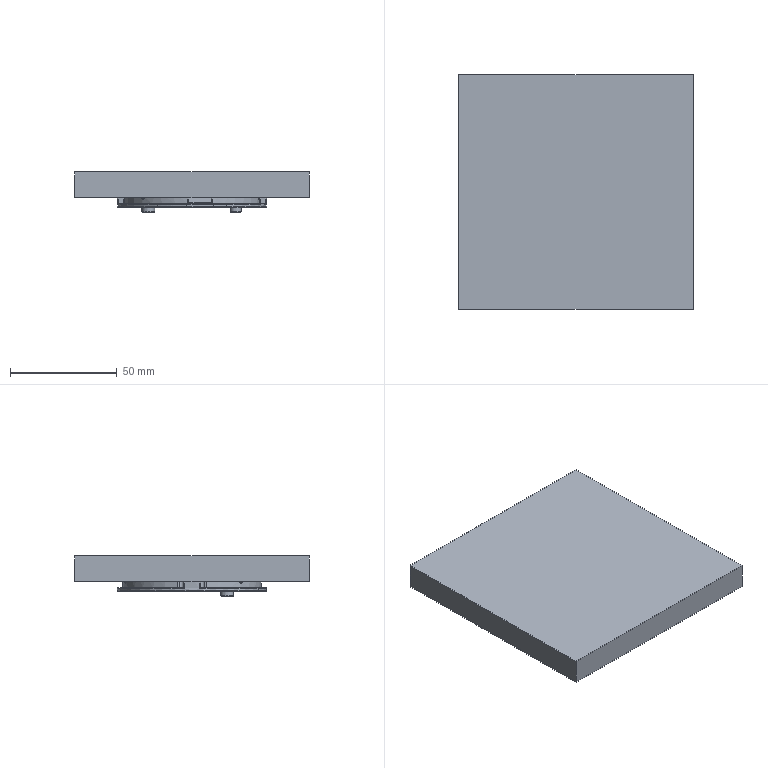NC program | NX | posted with a generic post | part box 110 x 110 x 18.8 mm
Lines 3402 to 4286 of 9447:
(CAVITY_MILL_COPY_1_COPY , TOOL : D3)
N6784 T17 M6
N6786 G54
N6788 G17 G0 G90 X-34.29 Y3.742 S9500 M3
N6790 G43 Z30. H17
N6792 Z-4.25
N6794 G94 G1 Z-5.25 F1000.
N6796 G3 X-33.488 Y4.304 R1.
N6798 G2 X-32.872 Y5.112 R2.5 F1100.
N6800 X-33.214 Y6.069 R2.5
N6802 G3 X-33.807 Y6.848 R1.
N6804 G1 Z-4.25
N6806 G0 X-34.29 Y3.742 Z-4.5
N6808 G1 Z-5.5 F1000.
N6810 G3 X-33.488 Y4.304 R1.
N6812 G2 X-32.872 Y5.112 R2.5 F1100.
N6814 X-33.214 Y6.069 R2.5
N6816 G3 X-33.807 Y6.848 R1.
N6818 G1 Z-4.5
N6820 G0 X-34.29 Y3.742 Z-4.75
N6822 G1 Z-5.75 F1000.
N6824 G3 X-33.488 Y4.304 R1.
N6826 G2 X-32.872 Y5.112 R2.5 F1100.
N6828 X-33.214 Y6.069 R2.5
N6830 G3 X-33.807 Y6.848 R1.
N6832 G1 Z-4.75
N6834 G0 X-34.29 Y3.742 Z-5.
N6836 G1 Z-6. F1000.
N6838 G3 X-33.488 Y4.304 R1.
N6840 G2 X-32.872 Y5.112 R2.5 F1100.
N6842 X-33.214 Y6.069 R2.5
N6844 G3 X-33.807 Y6.848 R1.
N6846 G1 Z-5.
N6848 G0 X-34.29 Y3.742 Z-5.25
N6850 G1 Z-6.25 F1000.
N6852 G3 X-33.488 Y4.304 R1.
N6854 G2 X-32.872 Y5.112 R2.5 F1100.
N6856 X-33.214 Y6.069 R2.5
N6858 G3 X-33.807 Y6.848 R1.
N6860 G1 Z-5.25
N6862 G0 X-34.29 Y3.742 Z-5.5
N6864 G1 Z-6.5 F1000.
N6866 G3 X-33.488 Y4.304 R1.
N6868 G2 X-32.872 Y5.112 R2.5 F1100.
N6870 X-33.214 Y6.069 R2.5
N6872 G3 X-33.807 Y6.848 R1.
N6874 G1 Z-5.5
N6876 G0 X-34.29 Y3.742 Z-5.75
N6878 G1 Z-6.75 F1000.
N6880 G3 X-33.488 Y4.304 R1.
N6882 G2 X-32.872 Y5.112 R2.5 F1100.
N6884 X-33.214 Y6.069 R2.5
N6886 G3 X-33.807 Y6.848 R1.
N6888 G1 Z-5.75
N6890 G0 X-34.29 Y3.742 Z-6.
N6892 G1 Z-7. F1000.
N6894 G3 X-33.488 Y4.304 R1.
N6896 G2 X-32.872 Y5.112 R2.5 F1100.
N6898 X-33.214 Y6.069 R2.5
N6900 G3 X-33.807 Y6.848 R1.
N6902 G1 Z-6.
N6904 G0 X-34.29 Y3.742 Z-6.25
N6906 G1 Z-7.25 F1000.
N6908 G3 X-33.488 Y4.304 R1.
N6910 G2 X-32.872 Y5.112 R2.5 F1100.
N6912 X-33.214 Y6.069 R2.5
N6914 G3 X-33.807 Y6.848 R1.
N6916 G1 Z-6.25
N6918 G0 X-34.29 Y3.742 Z-6.5
N6920 G1 Z-7.5 F1000.
N6922 G3 X-33.488 Y4.304 R1.
N6924 G2 X-32.872 Y5.112 R2.5 F1100.
N6926 X-33.214 Y6.069 R2.5
N6928 G3 X-33.807 Y6.848 R1.
N6930 G1 Z-6.5
N6932 G0 X-34.29 Y3.742 Z-6.75
N6934 G1 Z-7.75 F1000.
N6936 G3 X-33.488 Y4.304 R1.
N6938 G2 X-32.872 Y5.112 R2.5 F1100.
N6940 X-33.214 Y6.069 R2.5
N6942 G3 X-33.807 Y6.848 R1.
N6944 G1 Z-6.75
N6946 G0 X-34.29 Y3.742 Z-7.
N6948 G1 Z-8. F1000.
N6950 G3 X-33.488 Y4.304 R1.
N6952 G2 X-32.872 Y5.112 R2.5 F1100.
N6954 X-33.214 Y6.069 R2.5
N6956 G3 X-33.807 Y6.848 R1.
N6958 G1 Z-7.
N6960 G0 X-34.29 Y3.742 Z-7.25
N6962 G1 Z-8.25 F1000.
N6964 G3 X-33.488 Y4.304 R1.
N6966 G2 X-32.872 Y5.112 R2.5 F1100.
N6968 X-33.214 Y6.069 R2.5
N6970 G3 X-33.807 Y6.848 R1.
N6972 G1 Z-7.25
N6974 G0 X-34.29 Y3.742 Z-7.5
N6976 G1 Z-8.5 F1000.
N6978 G3 X-33.488 Y4.304 R1.
N6980 G2 X-32.872 Y5.112 R2.5 F1100.
N6982 X-33.214 Y6.069 R2.5
N6984 G3 X-33.807 Y6.848 R1.
N6986 G1 Z-7.5
N6988 G0 X-34.29 Y3.742 Z-7.75
N6990 G1 Z-8.75 F1000.
N6992 G3 X-33.488 Y4.304 R1.
N6994 G2 X-32.872 Y5.112 R2.5 F1100.
N6996 X-33.214 Y6.069 R2.5
N6998 G3 X-33.807 Y6.848 R1.
N7000 G1 Z-7.75
N7002 G0 X-34.29 Y3.742 Z-8.
N7004 G1 Z-9. F1000.
N7006 G3 X-33.488 Y4.304 R1.
N7008 G2 X-32.872 Y5.112 R2.5 F1100.
N7010 X-33.214 Y6.069 R2.5
N7012 G3 X-33.807 Y6.848 R1.
N7014 G1 Z-8.
N7016 G0 X-35.784 Y5.65 Z-8.25
N7018 G1 Z-9.25 F1000.
N7020 G3 X-34.851 Y5.429 R1.
N7022 G2 X-34.322 Y5.5 R2. F1100.
N7024 G1 X-33.065
N7026 G2 X-33.185 Y6.925 R2.5
N7028 G1 X-33.147 Y7.106
N7030 G3 X-33.454 Y8.058 R1.
N7032 G1 X-33.529 Y8.126
N7034 Z-8.25
N7036 G0 X-35.784 Y5.65 Z-8.5
N7038 G1 Z-9.5 F1000.
N7040 G3 X-34.851 Y5.429 R1.
N7042 G2 X-34.322 Y5.5 R2. F1100.
N7044 G1 X-33.065
N7046 G2 X-33.185 Y6.925 R2.5
N7048 G1 X-33.147 Y7.106
N7050 G3 X-33.454 Y8.058 R1.
N7052 G1 X-33.529 Y8.126
N7054 Z-8.5
N7056 G0 X-35.784 Y5.65 Z-8.75
N7058 G1 Z-9.75 F1000.
N7060 G3 X-34.851 Y5.429 R1.
N7062 G2 X-34.322 Y5.5 R2. F1100.
N7064 G1 X-33.065
N7066 G2 X-33.185 Y6.925 R2.5
N7068 G1 X-33.147 Y7.106
N7070 G3 X-33.454 Y8.058 R1.
N7072 G1 X-33.529 Y8.126
N7074 Z-8.75
N7076 G0 X-35.784 Y5.65 Z-9.
N7078 G1 Z-10. F1000.
N7080 G3 X-34.851 Y5.429 R1.
N7082 G2 X-34.322 Y5.5 R2. F1100.
N7084 G1 X-33.065
N7086 G2 X-33.185 Y6.925 R2.5
N7088 G1 X-33.147 Y7.106
N7090 G3 X-33.454 Y8.058 R1.
N7092 G1 X-33.529 Y8.126
N7094 Z-9.
N7096 G0 X-35.784 Y5.65 Z-9.25
N7098 G1 Z-10.25 F1000.
N7100 G3 X-34.851 Y5.429 R1.
N7102 G2 X-34.322 Y5.5 R2. F1100.
N7104 G1 X-33.065
N7106 G2 X-33.185 Y6.925 R2.5
N7108 G1 X-33.147 Y7.106
N7110 G3 X-33.454 Y8.058 R1.
N7112 G1 X-33.529 Y8.126
N7114 Z-9.25
N7116 G0 X-35.784 Y5.65 Z-9.5
N7118 G1 Z-10.5 F1000.
N7120 G3 X-34.851 Y5.429 R1.
N7122 G2 X-34.322 Y5.5 R2. F1100.
N7124 G1 X-33.065
N7126 G2 X-33.185 Y6.925 R2.5
N7128 G1 X-33.147 Y7.106
N7130 G3 X-33.454 Y8.058 R1.
N7132 G1 X-33.529 Y8.126
N7134 Z-9.5
N7136 G0 X-35.784 Y5.65 Z-9.75
N7138 G1 Z-10.75 F1000.
N7140 G3 X-34.851 Y5.429 R1.
N7142 G2 X-34.322 Y5.5 R2. F1100.
N7144 G1 X-33.065
N7146 G2 X-33.185 Y6.925 R2.5
N7148 G1 X-33.147 Y7.106
N7150 G3 X-33.454 Y8.058 R1.
N7152 G1 X-33.529 Y8.126
N7154 Z-9.75
N7156 G0 X-35.784 Y5.65 Z-10.
N7158 G1 Z-11. F1000.
N7160 G3 X-34.851 Y5.429 R1.
N7162 G2 X-34.322 Y5.5 R2. F1100.
N7164 G1 X-33.065
N7166 G2 X-33.185 Y6.925 R2.5
N7168 G1 X-33.147 Y7.106
N7170 G3 X-33.454 Y8.058 R1.
N7172 G1 X-33.529 Y8.126
N7174 Z-10.
N7176 G0 X-35.784 Y5.65 Z-10.25
N7178 G1 Z-11.25 F1000.
N7180 G3 X-34.851 Y5.429 R1.
N7182 G2 X-34.322 Y5.5 R2. F1100.
N7184 G1 X-33.065
N7186 G2 X-33.185 Y6.925 R2.5
N7188 G1 X-33.147 Y7.106
N7190 G3 X-33.454 Y8.058 R1.
N7192 G1 X-33.529 Y8.126
N7194 Z-10.25
N7196 G0 X-35.784 Y5.65 Z-10.5
N7198 G1 Z-11.5 F1000.
N7200 G3 X-34.851 Y5.429 R1.
N7202 G2 X-34.322 Y5.5 R2. F1100.
N7204 G1 X-33.065
N7206 G2 X-33.185 Y6.925 R2.5
N7208 G1 X-33.147 Y7.106
N7210 G3 X-33.454 Y8.058 R1.
N7212 G1 X-33.529 Y8.126
N7214 Z-10.5
N7216 G0 X-35.784 Y5.65 Z-10.75
N7218 G1 Z-11.75 F1000.
N7220 G3 X-34.851 Y5.429 R1.
N7222 G2 X-34.322 Y5.5 R2. F1100.
N7224 G1 X-33.065
N7226 G2 X-33.185 Y6.925 R2.5
N7228 G1 X-33.147 Y7.106
N7230 G3 X-33.454 Y8.058 R1.
N7232 G1 X-33.529 Y8.126
N7234 Z-10.75
N7236 G0 X-35.784 Y5.65 Z-11.
N7238 G1 Z-12. F1000.
N7240 G3 X-34.851 Y5.429 R1.
N7242 G2 X-34.322 Y5.5 R2. F1100.
N7244 G1 X-33.065
N7246 G2 X-33.185 Y6.925 R2.5
N7248 G1 X-33.147 Y7.106
N7250 G3 X-33.454 Y8.058 R1.
N7252 G1 X-33.529 Y8.126
N7254 Z-11.
N7256 G0 Z30.
N7258 X-33.807 Y-6.848
N7260 Z-4.25
N7262 G1 Z-5.25 F1000.
N7264 G3 X-33.214 Y-6.069 R1.
N7266 G2 X-32.872 Y-5.112 R2.5 F1100.
N7268 X-33.488 Y-4.304 R2.5
N7270 G3 X-34.29 Y-3.742 R1.
N7272 G1 Z-4.25
N7274 G0 X-33.807 Y-6.848 Z-4.5
N7276 G1 Z-5.5 F1000.
N7278 G3 X-33.214 Y-6.069 R1.
N7280 G2 X-32.872 Y-5.112 R2.5 F1100.
N7282 X-33.488 Y-4.304 R2.5
N7284 G3 X-34.29 Y-3.742 R1.
N7286 G1 Z-4.5
N7288 G0 X-33.807 Y-6.848 Z-4.75
N7290 G1 Z-5.75 F1000.
N7292 G3 X-33.214 Y-6.069 R1.
N7294 G2 X-32.872 Y-5.112 R2.5 F1100.
N7296 X-33.488 Y-4.304 R2.5
N7298 G3 X-34.29 Y-3.742 R1.
N7300 G1 Z-4.75
N7302 G0 X-33.807 Y-6.848 Z-5.
N7304 G1 Z-6. F1000.
N7306 G3 X-33.214 Y-6.069 R1.
N7308 G2 X-32.872 Y-5.112 R2.5 F1100.
N7310 X-33.488 Y-4.304 R2.5
N7312 G3 X-34.291 Y-3.741 R1.
N7314 G1 Z-5.
N7316 G0 X-33.807 Y-6.848 Z-5.25
N7318 G1 Z-6.25 F1000.
N7320 G3 X-33.214 Y-6.069 R1.
N7322 G2 X-32.872 Y-5.112 R2.5 F1100.
N7324 X-33.488 Y-4.304 R2.5
N7326 G3 X-34.29 Y-3.742 R1.
N7328 G1 Z-5.25
N7330 G0 X-33.807 Y-6.848 Z-5.5
N7332 G1 Z-6.5 F1000.
N7334 G3 X-33.214 Y-6.069 R1.
N7336 G2 X-32.872 Y-5.112 R2.5 F1100.
N7338 X-33.488 Y-4.304 R2.5
N7340 G3 X-34.29 Y-3.742 R1.
N7342 G1 Z-5.5
N7344 G0 X-33.807 Y-6.848 Z-5.75
N7346 G1 Z-6.75 F1000.
N7348 G3 X-33.214 Y-6.069 R1.
N7350 G2 X-32.872 Y-5.112 R2.5 F1100.
N7352 X-33.488 Y-4.304 R2.5
N7354 G3 X-34.29 Y-3.742 R1.
N7356 G1 Z-5.75
N7358 G0 X-33.807 Y-6.848 Z-6.
N7360 G1 Z-7. F1000.
N7362 G3 X-33.214 Y-6.069 R1.
N7364 G2 X-32.872 Y-5.112 R2.5 F1100.
N7366 X-33.488 Y-4.304 R2.5
N7368 G3 X-34.29 Y-3.742 R1.
N7370 G1 Z-6.
N7372 G0 X-33.807 Y-6.848 Z-6.25
N7374 G1 Z-7.25 F1000.
N7376 G3 X-33.214 Y-6.069 R1.
N7378 G2 X-32.872 Y-5.112 R2.5 F1100.
N7380 X-33.488 Y-4.304 R2.5
N7382 G3 X-34.29 Y-3.742 R1.
N7384 G1 Z-6.25
N7386 G0 X-33.807 Y-6.848 Z-6.5
N7388 G1 Z-7.5 F1000.
N7390 G3 X-33.214 Y-6.069 R1.
N7392 G2 X-32.872 Y-5.112 R2.5 F1100.
N7394 X-33.488 Y-4.304 R2.5
N7396 G3 X-34.29 Y-3.742 R1.
N7398 G1 Z-6.5
N7400 G0 X-33.807 Y-6.848 Z-6.75
N7402 G1 Z-7.75 F1000.
N7404 G3 X-33.214 Y-6.069 R1.
N7406 G2 X-32.872 Y-5.112 R2.5 F1100.
N7408 X-33.488 Y-4.304 R2.5
N7410 G3 X-34.29 Y-3.742 R1.
N7412 G1 Z-6.75
N7414 G0 X-33.807 Y-6.848 Z-7.
N7416 G1 Z-8. F1000.
N7418 G3 X-33.214 Y-6.069 R1.
N7420 G2 X-32.872 Y-5.112 R2.5 F1100.
N7422 X-33.488 Y-4.304 R2.5
N7424 G3 X-34.29 Y-3.742 R1.
N7426 G1 Z-7.
N7428 G0 X-33.807 Y-6.848 Z-7.25
N7430 G1 Z-8.25 F1000.
N7432 G3 X-33.214 Y-6.069 R1.
N7434 G2 X-32.872 Y-5.112 R2.5 F1100.
N7436 X-33.488 Y-4.304 R2.5
N7438 G3 X-34.29 Y-3.742 R1.
N7440 G1 Z-7.25
N7442 G0 X-33.807 Y-6.848 Z-7.5
N7444 G1 Z-8.5 F1000.
N7446 G3 X-33.214 Y-6.069 R1.
N7448 G2 X-32.872 Y-5.112 R2.5 F1100.
N7450 X-33.488 Y-4.304 R2.5
N7452 G3 X-34.29 Y-3.742 R1.
N7454 G1 Z-7.5
N7456 G0 X-33.807 Y-6.848 Z-7.75
N7458 G1 Z-8.75 F1000.
N7460 G3 X-33.214 Y-6.069 R1.
N7462 G2 X-32.872 Y-5.112 R2.5 F1100.
N7464 X-33.488 Y-4.304 R2.5
N7466 G3 X-34.29 Y-3.742 R1.
N7468 G1 Z-7.75
N7470 G0 X-33.807 Y-6.848 Z-8.
N7472 G1 Z-9. F1000.
N7474 G3 X-33.214 Y-6.069 R1.
N7476 G2 X-32.872 Y-5.112 R2.5 F1100.
N7478 X-33.488 Y-4.304 R2.5
N7480 G3 X-34.29 Y-3.741 R1.
N7482 G1 Z-8.
N7484 G0 X-33.529 Y-8.126 Z-8.25
N7486 G1 Z-9.25 F1000.
N7488 X-33.454 Y-8.058
N7490 G3 X-33.147 Y-7.106 R1.
N7492 G1 X-33.185 Y-6.925 F1100.
N7494 G2 X-33.065 Y-5.5 R2.5
N7496 G1 X-34.322
N7498 G2 X-34.851 Y-5.429 R2.
N7500 G3 X-35.784 Y-5.65 R1.
N7502 G1 Z-8.25
N7504 G0 X-33.529 Y-8.126 Z-8.5
N7506 G1 Z-9.5 F1000.
N7508 X-33.454 Y-8.058
N7510 G3 X-33.147 Y-7.106 R1.
N7512 G1 X-33.185 Y-6.925 F1100.
N7514 G2 X-33.065 Y-5.5 R2.5
N7516 G1 X-34.322
N7518 G2 X-34.851 Y-5.429 R2.
N7520 G3 X-35.784 Y-5.65 R1.
N7522 G1 Z-8.5
N7524 G0 X-33.529 Y-8.126 Z-8.75
N7526 G1 Z-9.75 F1000.
N7528 X-33.454 Y-8.058
N7530 G3 X-33.147 Y-7.106 R1.
N7532 G1 X-33.185 Y-6.925 F1100.
N7534 G2 X-33.065 Y-5.5 R2.5
N7536 G1 X-34.322
N7538 G2 X-34.851 Y-5.429 R2.
N7540 G3 X-35.784 Y-5.65 R1.
N7542 G1 Z-8.75
N7544 G0 X-33.529 Y-8.126 Z-9.
N7546 G1 Z-10. F1000.
N7548 X-33.454 Y-8.058
N7550 G3 X-33.147 Y-7.106 R1.
N7552 G1 X-33.185 Y-6.925 F1100.
N7554 G2 X-33.065 Y-5.5 R2.5
N7556 G1 X-34.322
N7558 G2 X-34.851 Y-5.429 R2.
N7560 G3 X-35.784 Y-5.65 R1.
N7562 G1 Z-9.
N7564 G0 X-33.529 Y-8.126 Z-9.25
N7566 G1 Z-10.25 F1000.
N7568 X-33.454 Y-8.058
N7570 G3 X-33.147 Y-7.106 R1.
N7572 G1 X-33.185 Y-6.925 F1100.
N7574 G2 X-33.065 Y-5.5 R2.5
N7576 G1 X-34.322
N7578 G2 X-34.851 Y-5.429 R2.
N7580 G3 X-35.784 Y-5.65 R1.
N7582 G1 Z-9.25
N7584 G0 X-33.529 Y-8.126 Z-9.5
N7586 G1 Z-10.5 F1000.
N7588 X-33.454 Y-8.058
N7590 G3 X-33.147 Y-7.106 R1.
N7592 G1 X-33.185 Y-6.925 F1100.
N7594 G2 X-33.065 Y-5.5 R2.5
N7596 G1 X-34.322
N7598 G2 X-34.851 Y-5.429 R2.
N7600 G3 X-35.784 Y-5.65 R1.
N7602 G1 Z-9.5
N7604 G0 X-33.529 Y-8.126 Z-9.75
N7606 G1 Z-10.75 F1000.
N7608 X-33.454 Y-8.058
N7610 G3 X-33.147 Y-7.106 R1.
N7612 G1 X-33.185 Y-6.925 F1100.
N7614 G2 X-33.065 Y-5.5 R2.5
N7616 G1 X-34.322
N7618 G2 X-34.851 Y-5.429 R2.
N7620 G3 X-35.784 Y-5.65 R1.
N7622 G1 Z-9.75
N7624 G0 X-33.529 Y-8.126 Z-10.
N7626 G1 Z-11. F1000.
N7628 X-33.454 Y-8.058
N7630 G3 X-33.147 Y-7.106 R1.
N7632 G1 X-33.185 Y-6.925 F1100.
N7634 G2 X-33.065 Y-5.5 R2.5
N7636 G1 X-34.322
N7638 G2 X-34.851 Y-5.429 R2.
N7640 G3 X-35.784 Y-5.65 R1.
N7642 G1 Z-10.
N7644 G0 X-33.529 Y-8.126 Z-10.25
N7646 G1 Z-11.25 F1000.
N7648 X-33.454 Y-8.058
N7650 G3 X-33.147 Y-7.106 R1.
N7652 G1 X-33.185 Y-6.925 F1100.
N7654 G2 X-33.065 Y-5.5 R2.5
N7656 G1 X-34.322
N7658 G2 X-34.851 Y-5.429 R2.
N7660 G3 X-35.784 Y-5.65 R1.
N7662 G1 Z-10.25
N7664 G0 X-33.529 Y-8.126 Z-10.5
N7666 G1 Z-11.5 F1000.
N7668 X-33.454 Y-8.058
N7670 G3 X-33.147 Y-7.106 R1.
N7672 G1 X-33.185 Y-6.925 F1100.
N7674 G2 X-33.065 Y-5.5 R2.5
N7676 G1 X-34.322
N7678 G2 X-34.851 Y-5.429 R2.
N7680 G3 X-35.784 Y-5.65 R1.
N7682 G1 Z-10.5
N7684 G0 X-33.529 Y-8.126 Z-10.75
N7686 G1 Z-11.75 F1000.
N7688 X-33.454 Y-8.058
N7690 G3 X-33.147 Y-7.106 R1.
N7692 G1 X-33.185 Y-6.925 F1100.
N7694 G2 X-33.065 Y-5.5 R2.5
N7696 G1 X-34.322
N7698 G2 X-34.851 Y-5.429 R2.
N7700 G3 X-35.784 Y-5.65 R1.
N7702 G1 Z-10.75
N7704 G0 X-33.529 Y-8.126 Z-11.
N7706 G1 Z-12. F1000.
N7708 X-33.454 Y-8.058
N7710 G3 X-33.147 Y-7.106 R1.
N7712 G1 X-33.185 Y-6.925 F1100.
N7714 G2 X-33.065 Y-5.5 R2.5
N7716 G1 X-34.322
N7718 G2 X-34.851 Y-5.429 R2.
N7720 G3 X-35.784 Y-5.65 R1.
N7722 G1 Z-11.
N7724 G0 Z30.
N7726 X-24.498 Y-14.169
N7728 Z-4.25
N7730 G1 Z-5.25 F1000.
N7732 X-24.56 Y-14.286
N7734 G3 X-24.527 Y-15.286 R1.
N7736 X-23.81 Y-16.379 R28.9 F1100.
N7738 G2 X-22.711 Y-16.183 R2.5
N7740 G3 X-21.835 Y-15.745 R1.
N7742 G1 Z-4.25
N7744 G0 X-24.498 Y-14.169 Z-4.5
N7746 G1 Z-5.5 F1000.
N7748 X-24.56 Y-14.286
N7750 G3 X-24.527 Y-15.286 R1.
N7752 X-23.81 Y-16.379 R28.9 F1100.
N7754 G2 X-22.711 Y-16.183 R2.5
N7756 G3 X-21.835 Y-15.745 R1.
N7758 G1 Z-4.5
N7760 G0 X-24.498 Y-14.169 Z-4.75
N7762 G1 Z-5.75 F1000.
N7764 X-24.56 Y-14.286
N7766 G3 X-24.527 Y-15.286 R1.
N7768 X-23.81 Y-16.379 R28.9 F1100.
N7770 G2 X-22.711 Y-16.183 R2.5
N7772 G3 X-21.835 Y-15.745 R1.
N7774 G1 Z-4.75
N7776 G0 X-24.498 Y-14.169 Z-5.
N7778 G1 Z-6. F1000.
N7780 X-24.56 Y-14.286
N7782 G3 X-24.527 Y-15.286 R1.
N7784 X-23.81 Y-16.379 R28.9 F1100.
N7786 G2 X-22.711 Y-16.183 R2.5
N7788 G3 X-21.835 Y-15.745 R1.
N7790 G1 Z-5.
N7792 G0 X-24.498 Y-14.169 Z-5.25
N7794 G1 Z-6.25 F1000.
N7796 X-24.56 Y-14.286
N7798 G3 X-24.527 Y-15.286 R1.
N7800 X-23.81 Y-16.379 R28.9 F1100.
N7802 G2 X-22.711 Y-16.183 R2.5
N7804 G3 X-21.835 Y-15.745 R1.
N7806 G1 Z-5.25
N7808 G0 X-24.498 Y-14.169 Z-5.5
N7810 G1 Z-6.5 F1000.
N7812 X-24.56 Y-14.286
N7814 G3 X-24.527 Y-15.286 R1.
N7816 X-23.81 Y-16.379 R28.9 F1100.
N7818 G2 X-22.711 Y-16.183 R2.5
N7820 G3 X-21.835 Y-15.745 R1.
N7822 G1 Z-5.5
N7824 G0 X-24.498 Y-14.169 Z-5.75
N7826 G1 Z-6.75 F1000.
N7828 X-24.56 Y-14.286
N7830 G3 X-24.527 Y-15.286 R1.
N7832 X-23.81 Y-16.379 R28.9 F1100.
N7834 G2 X-22.711 Y-16.183 R2.5
N7836 G3 X-21.835 Y-15.745 R1.
N7838 G1 Z-5.75
N7840 G0 X-24.498 Y-14.169 Z-6.
N7842 G1 Z-7. F1000.
N7844 X-24.56 Y-14.286
N7846 G3 X-24.527 Y-15.286 R1.
N7848 X-23.81 Y-16.379 R28.9 F1100.
N7850 G2 X-22.711 Y-16.183 R2.5
N7852 G3 X-21.835 Y-15.745 R1.
N7854 G1 Z-6.
N7856 G0 X-24.498 Y-14.169 Z-6.25
N7858 G1 Z-7.25 F1000.
N7860 X-24.56 Y-14.286
N7862 G3 X-24.527 Y-15.286 R1.
N7864 X-23.81 Y-16.379 R28.9 F1100.
N7866 G2 X-22.711 Y-16.183 R2.5
N7868 G3 X-21.835 Y-15.745 R1.
N7870 G1 Z-6.25
N7872 G0 X-24.498 Y-14.169 Z-6.5
N7874 G1 Z-7.5 F1000.
N7876 X-24.56 Y-14.286
N7878 G3 X-24.527 Y-15.286 R1.
N7880 X-23.81 Y-16.379 R28.9 F1100.
N7882 G2 X-22.711 Y-16.183 R2.5
N7884 G3 X-21.835 Y-15.745 R1.
N7886 G1 Z-6.5
N7888 G0 X-24.498 Y-14.169 Z-6.75
N7890 G1 Z-7.75 F1000.
N7892 X-24.56 Y-14.286
N7894 G3 X-24.527 Y-15.286 R1.
N7896 X-23.81 Y-16.379 R28.9 F1100.
N7898 G2 X-22.711 Y-16.183 R2.5
N7900 G3 X-21.835 Y-15.745 R1.
N7902 G1 Z-6.75
N7904 G0 X-24.498 Y-14.169 Z-7.
N7906 G1 Z-8. F1000.
N7908 X-24.56 Y-14.286
N7910 G3 X-24.527 Y-15.286 R1.
N7912 X-23.81 Y-16.379 R28.9 F1100.
N7914 G2 X-22.711 Y-16.183 R2.5
N7916 G3 X-21.835 Y-15.745 R1.
N7918 G1 Z-7.
N7920 G0 X-24.498 Y-14.169 Z-7.25
N7922 G1 Z-8.25 F1000.
N7924 X-24.56 Y-14.286
N7926 G3 X-24.527 Y-15.286 R1.
N7928 X-23.81 Y-16.379 R28.9 F1100.
N7930 G2 X-22.711 Y-16.183 R2.5
N7932 G3 X-21.835 Y-15.745 R1.
N7934 G1 Z-7.25
N7936 G0 X-24.498 Y-14.169 Z-7.5
N7938 G1 Z-8.5 F1000.
N7940 X-24.56 Y-14.286
N7942 G3 X-24.527 Y-15.286 R1.
N7944 X-23.81 Y-16.379 R28.9 F1100.
N7946 G2 X-22.711 Y-16.183 R2.5
N7948 G3 X-21.835 Y-15.745 R1.
N7950 G1 Z-7.5
N7952 G0 X-24.498 Y-14.169 Z-7.75
N7954 G1 Z-8.75 F1000.
N7956 X-24.56 Y-14.286
N7958 G3 X-24.527 Y-15.286 R1.
N7960 X-23.81 Y-16.379 R28.9 F1100.
N7962 G2 X-22.711 Y-16.183 R2.5
N7964 G3 X-21.835 Y-15.745 R1.
N7966 G1 Z-7.75
N7968 G0 X-24.498 Y-14.169 Z-8.
N7970 G1 Z-9. F1000.
N7972 X-24.56 Y-14.286
N7974 G3 X-24.527 Y-15.286 R1.
N7976 X-23.81 Y-16.379 R28.9 F1100.
N7978 G2 X-22.711 Y-16.183 R2.5
N7980 G3 X-21.835 Y-15.745 R1.
N7982 G1 Z-8.
N7984 G0 X-24.498 Y-14.169 Z-8.25
N7986 G1 Z-9.25 F1000.
N7988 X-24.56 Y-14.286
N7990 G3 X-24.527 Y-15.286 R1.
N7992 X-23.81 Y-16.379 R28.9 F1100.
N7994 G2 X-22.711 Y-16.183 R2.5
N7996 G3 X-21.835 Y-15.745 R1.
N7998 G1 Z-8.25
N8000 G0 X-24.498 Y-14.169 Z-8.5
N8002 G1 Z-9.5 F1000.
N8004 X-24.56 Y-14.286
N8006 G3 X-24.527 Y-15.286 R1.
N8008 X-23.81 Y-16.379 R28.9 F1100.
N8010 G2 X-22.711 Y-16.183 R2.5
N8012 G3 X-21.835 Y-15.745 R1.
N8014 G1 Z-8.5
N8016 G0 X-24.498 Y-14.169 Z-8.75
N8018 G1 Z-9.75 F1000.
N8020 X-24.56 Y-14.286
N8022 G3 X-24.527 Y-15.286 R1.
N8024 X-23.81 Y-16.379 R28.9 F1100.
N8026 G2 X-22.711 Y-16.183 R2.5
N8028 G3 X-21.835 Y-15.745 R1.
N8030 G1 Z-8.75
N8032 G0 X-24.498 Y-14.169 Z-9.
N8034 G1 Z-10. F1000.
N8036 X-24.56 Y-14.286
N8038 G3 X-24.527 Y-15.286 R1.
N8040 X-23.81 Y-16.379 R28.9 F1100.
N8042 G2 X-22.711 Y-16.183 R2.5
N8044 G3 X-21.835 Y-15.745 R1.
N8046 G1 Z-9.
N8048 G0 X-24.498 Y-14.169 Z-9.25
N8050 G1 Z-10.25 F1000.
N8052 X-24.56 Y-14.286
N8054 G3 X-24.527 Y-15.286 R1.
N8056 X-23.81 Y-16.379 R28.9 F1100.
N8058 G2 X-22.711 Y-16.183 R2.5
N8060 G3 X-21.835 Y-15.745 R1.
N8062 G1 Z-9.25
N8064 G0 X-24.498 Y-14.169 Z-9.5
N8066 G1 Z-10.5 F1000.
N8068 X-24.56 Y-14.286
N8070 G3 X-24.527 Y-15.286 R1.
N8072 X-23.81 Y-16.379 R28.9 F1100.
N8074 G2 X-22.711 Y-16.183 R2.5
N8076 G3 X-21.835 Y-15.745 R1.
N8078 G1 Z-9.5
N8080 G0 X-24.498 Y-14.169 Z-9.75
N8082 G1 Z-10.75 F1000.
N8084 X-24.56 Y-14.286
N8086 G3 X-24.527 Y-15.286 R1.
N8088 X-23.81 Y-16.379 R28.9 F1100.
N8090 G2 X-22.711 Y-16.183 R2.5
N8092 G3 X-21.835 Y-15.745 R1.
N8094 G1 Z-9.75
N8096 G0 X-24.498 Y-14.169 Z-10.
N8098 G1 Z-11. F1000.
N8100 X-24.56 Y-14.286
N8102 G3 X-24.527 Y-15.286 R1.
N8104 X-23.81 Y-16.379 R28.9 F1100.
N8106 G2 X-22.711 Y-16.183 R2.5
N8108 G3 X-21.835 Y-15.745 R1.
N8110 G1 Z-10.
N8112 G0 X-24.498 Y-14.169 Z-10.25
N8114 G1 Z-11.25 F1000.
N8116 X-24.56 Y-14.286
N8118 G3 X-24.527 Y-15.286 R1.
N8120 X-23.81 Y-16.379 R28.9 F1100.
N8122 G2 X-22.711 Y-16.183 R2.5
N8124 G3 X-21.835 Y-15.745 R1.
N8126 G1 Z-10.25
N8128 G0 X-24.498 Y-14.169 Z-10.5
N8130 G1 Z-11.5 F1000.
N8132 X-24.56 Y-14.286
N8134 G3 X-24.527 Y-15.286 R1.
N8136 X-23.81 Y-16.379 R28.9 F1100.
N8138 G2 X-22.711 Y-16.183 R2.5
N8140 G3 X-21.835 Y-15.745 R1.
N8142 G1 Z-10.5
N8144 G0 Z30.
N8146 X-15.745 Y-21.835
N8148 Z-4.25
N8150 G1 Z-5.25 F1000.
N8152 G3 X-16.183 Y-22.711 R1.
N8154 G2 X-16.379 Y-23.81 R2.5 F1100.
N8156 G3 X-15.286 Y-24.527 R28.9
N8158 X-14.286 Y-24.56 R1.
N8160 G1 X-14.169 Y-24.498
N8162 Z-4.25
N8164 G0 X-15.745 Y-21.835 Z-4.5
N8166 G1 Z-5.5 F1000.
N8168 G3 X-16.183 Y-22.711 R1.
N8170 G2 X-16.379 Y-23.81 R2.5 F1100.
N8172 G3 X-15.286 Y-24.527 R28.9
N8174 X-14.286 Y-24.56 R1.
N8176 G1 X-14.169 Y-24.498
N8178 Z-4.5
N8180 G0 X-15.745 Y-21.835 Z-4.75
N8182 G1 Z-5.75 F1000.
N8184 G3 X-16.183 Y-22.711 R1.
N8186 G2 X-16.379 Y-23.81 R2.5 F1100.
N8188 G3 X-15.286 Y-24.527 R28.9
N8190 X-14.286 Y-24.56 R1.
N8192 G1 X-14.169 Y-24.498
N8194 Z-4.75
N8196 G0 X-15.745 Y-21.835 Z-5.
N8198 G1 Z-6. F1000.
N8200 G3 X-16.183 Y-22.711 R1.
N8202 G2 X-16.379 Y-23.81 R2.5 F1100.
N8204 G3 X-15.286 Y-24.527 R28.9
N8206 X-14.286 Y-24.56 R1.
N8208 G1 X-14.169 Y-24.498
N8210 Z-5.
N8212 G0 X-15.745 Y-21.835 Z-5.25
N8214 G1 Z-6.25 F1000.
N8216 G3 X-16.183 Y-22.711 R1.
N8218 G2 X-16.379 Y-23.81 R2.5 F1100.
N8220 G3 X-15.286 Y-24.527 R28.9
N8222 X-14.286 Y-24.56 R1.
N8224 G1 X-14.169 Y-24.498
N8226 Z-5.25
N8228 G0 X-15.745 Y-21.835 Z-5.5
N8230 G1 Z-6.5 F1000.
N8232 G3 X-16.183 Y-22.711 R1.
N8234 G2 X-16.379 Y-23.81 R2.5 F1100.
N8236 G3 X-15.286 Y-24.527 R28.9
N8238 X-14.286 Y-24.56 R1.
N8240 G1 X-14.169 Y-24.498
N8242 Z-5.5
N8244 G0 X-15.745 Y-21.835 Z-5.75
N8246 G1 Z-6.75 F1000.
N8248 G3 X-16.183 Y-22.711 R1.
N8250 G2 X-16.379 Y-23.81 R2.5 F1100.
N8252 G3 X-15.286 Y-24.527 R28.9
N8254 X-14.286 Y-24.56 R1.
N8256 G1 X-14.169 Y-24.498
N8258 Z-5.75
N8260 G0 X-15.745 Y-21.835 Z-6.
N8262 G1 Z-7. F1000.
N8264 G3 X-16.183 Y-22.711 R1.
N8266 G2 X-16.379 Y-23.81 R2.5 F1100.
N8268 G3 X-15.286 Y-24.527 R28.9
N8270 X-14.286 Y-24.56 R1.
N8272 G1 X-14.169 Y-24.498
N8274 Z-6.
N8276 G0 X-15.745 Y-21.835 Z-6.25
N8278 G1 Z-7.25 F1000.
N8280 G3 X-16.183 Y-22.711 R1.
N8282 G2 X-16.379 Y-23.81 R2.5 F1100.
N8284 G3 X-15.286 Y-24.527 R28.9
N8286 X-14.286 Y-24.56 R1.
N8288 G1 X-14.169 Y-24.498
N8290 Z-6.25
N8292 G0 X-15.745 Y-21.835 Z-6.5
N8294 G1 Z-7.5 F1000.
N8296 G3 X-16.183 Y-22.711 R1.
N8298 G2 X-16.379 Y-23.81 R2.5 F1100.
N8300 G3 X-15.286 Y-24.527 R28.9
N8302 X-14.286 Y-24.56 R1.
N8304 G1 X-14.169 Y-24.498
N8306 Z-6.5
N8308 G0 X-15.745 Y-21.835 Z-6.75
N8310 G1 Z-7.75 F1000.
N8312 G3 X-16.183 Y-22.711 R1.
N8314 G2 X-16.379 Y-23.81 R2.5 F1100.
N8316 G3 X-15.286 Y-24.527 R28.9
N8318 X-14.286 Y-24.56 R1.
N8320 G1 X-14.169 Y-24.498
N8322 Z-6.75
N8324 G0 X-15.745 Y-21.835 Z-7.
N8326 G1 Z-8. F1000.
N8328 G3 X-16.183 Y-22.711 R1.
N8330 G2 X-16.379 Y-23.81 R2.5 F1100.
N8332 G3 X-15.286 Y-24.527 R28.9
N8334 X-14.286 Y-24.56 R1.
N8336 G1 X-14.169 Y-24.498
N8338 Z-7.
N8340 G0 X-15.745 Y-21.835 Z-7.25
N8342 G1 Z-8.25 F1000.
N8344 G3 X-16.183 Y-22.711 R1.
N8346 G2 X-16.379 Y-23.81 R2.5 F1100.
N8348 G3 X-15.286 Y-24.527 R28.9
N8350 X-14.286 Y-24.56 R1.
N8352 G1 X-14.169 Y-24.498
N8354 Z-7.25
N8356 G0 X-15.745 Y-21.835 Z-7.5
N8358 G1 Z-8.5 F1000.
N8360 G3 X-16.183 Y-22.711 R1.
N8362 G2 X-16.379 Y-23.81 R2.5 F1100.
N8364 G3 X-15.286 Y-24.527 R28.9
N8366 X-14.286 Y-24.56 R1.
N8368 G1 X-14.169 Y-24.498
N8370 Z-7.5
N8372 G0 X-15.745 Y-21.835 Z-7.75
N8374 G1 Z-8.75 F1000.
N8376 G3 X-16.183 Y-22.711 R1.
N8378 G2 X-16.379 Y-23.81 R2.5 F1100.
N8380 G3 X-15.286 Y-24.527 R28.9
N8382 X-14.286 Y-24.56 R1.
N8384 G1 X-14.169 Y-24.498
N8386 Z-7.75
N8388 G0 X-15.745 Y-21.835 Z-8.
N8390 G1 Z-9. F1000.
N8392 G3 X-16.183 Y-22.711 R1.
N8394 G2 X-16.379 Y-23.81 R2.5 F1100.
N8396 G3 X-15.286 Y-24.527 R28.9
N8398 X-14.286 Y-24.56 R1.
N8400 G1 X-14.169 Y-24.498
N8402 Z-8.
N8404 G0 X-15.745 Y-21.835 Z-8.25
N8406 G1 Z-9.25 F1000.
N8408 G3 X-16.183 Y-22.711 R1.
N8410 G2 X-16.379 Y-23.81 R2.5 F1100.
N8412 G3 X-15.286 Y-24.527 R28.9
N8414 X-14.286 Y-24.56 R1.
N8416 G1 X-14.169 Y-24.498
N8418 Z-8.25
N8420 G0 X-15.745 Y-21.835 Z-8.5
N8422 G1 Z-9.5 F1000.
N8424 G3 X-16.183 Y-22.711 R1.
N8426 G2 X-16.379 Y-23.81 R2.5 F1100.
N8428 G3 X-15.286 Y-24.527 R28.9
N8430 X-14.286 Y-24.56 R1.
N8432 G1 X-14.169 Y-24.498
N8434 Z-8.5
N8436 G0 X-15.745 Y-21.835 Z-8.75
N8438 G1 Z-9.75 F1000.
N8440 G3 X-16.183 Y-22.711 R1.
N8442 G2 X-16.379 Y-23.81 R2.5 F1100.
N8444 G3 X-15.286 Y-24.527 R28.9
N8446 X-14.286 Y-24.56 R1.
N8448 G1 X-14.169 Y-24.498
N8450 Z-8.75
N8452 G0 X-15.745 Y-21.835 Z-9.
N8454 G1 Z-10. F1000.
N8456 G3 X-16.183 Y-22.711 R1.
N8458 G2 X-16.379 Y-23.81 R2.5 F1100.
N8460 G3 X-15.286 Y-24.527 R28.9
N8462 X-14.286 Y-24.56 R1.
N8464 G1 X-14.169 Y-24.498
N8466 Z-9.
N8468 G0 X-15.745 Y-21.835 Z-9.25
N8470 G1 Z-10.25 F1000.
N8472 G3 X-16.183 Y-22.711 R1.
N8474 G2 X-16.379 Y-23.81 R2.5 F1100.
N8476 G3 X-15.286 Y-24.527 R28.9
N8478 X-14.286 Y-24.56 R1.
N8480 G1 X-14.169 Y-24.498
N8482 Z-9.25
N8484 G0 X-15.745 Y-21.835 Z-9.5
N8486 G1 Z-10.5 F1000.
N8488 G3 X-16.183 Y-22.711 R1.
N8490 G2 X-16.379 Y-23.81 R2.5 F1100.
N8492 G3 X-15.286 Y-24.527 R28.9
N8494 X-14.286 Y-24.56 R1.
N8496 G1 X-14.169 Y-24.498
N8498 Z-9.5
N8500 G0 X-15.745 Y-21.835 Z-9.75
N8502 G1 Z-10.75 F1000.
N8504 G3 X-16.183 Y-22.711 R1.
N8506 G2 X-16.379 Y-23.81 R2.5 F1100.
N8508 G3 X-15.286 Y-24.527 R28.9
N8510 X-14.286 Y-24.56 R1.
N8512 G1 X-14.169 Y-24.498
N8514 Z-9.75
N8516 G0 X-15.745 Y-21.835 Z-10.
N8518 G1 Z-11. F1000.
N8520 G3 X-16.183 Y-22.711 R1.
N8522 G2 X-16.379 Y-23.81 R2.5 F1100.
N8524 G3 X-15.286 Y-24.527 R28.9
N8526 X-14.286 Y-24.56 R1.
N8528 G1 X-14.169 Y-24.498
N8530 Z-10.
N8532 G0 X-15.745 Y-21.835 Z-10.25
N8534 G1 Z-11.25 F1000.
N8536 G3 X-16.183 Y-22.711 R1.
N8538 G2 X-16.379 Y-23.81 R2.5 F1100.
N8540 G3 X-15.286 Y-24.527 R28.9
N8542 X-14.286 Y-24.56 R1.
N8544 G1 X-14.169 Y-24.498
N8546 Z-10.25